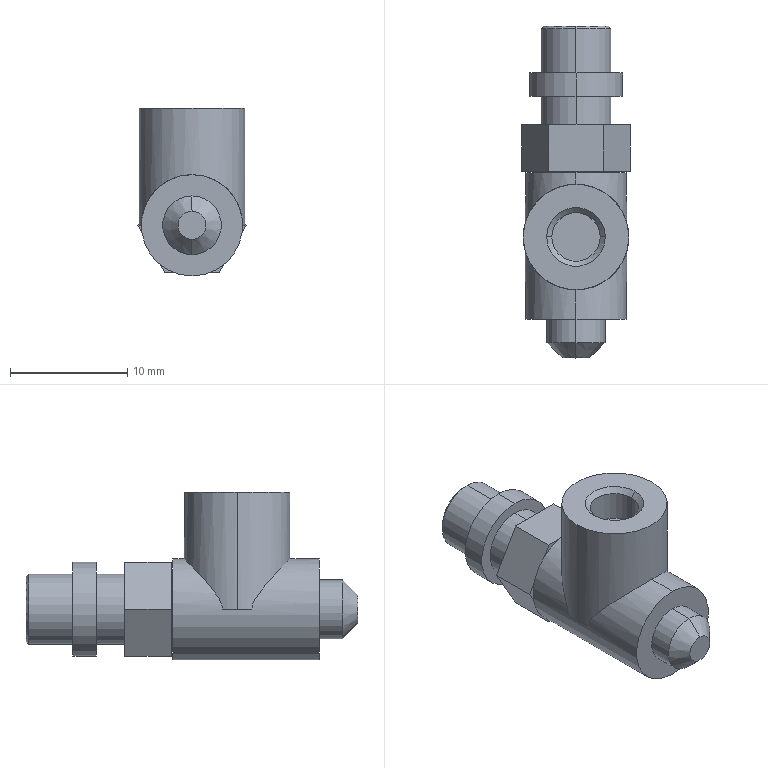Part | NX | features BREP 1 | 1 solid | 40 faces | box 9.238 x 28.3 x 14.32 mm | volume 1659 mm3 | plane 18 | cylinder 16 | cone 6 | commonest cylinder face diameters 6 x6 4.134 x2 5 x2 8 x2 8.64 x2 9 x2
STEP:
#1=CARTESIAN_POINT('',(0.,-7.,4.32));
#2=VERTEX_POINT('',#1);
#3=CARTESIAN_POINT('',(0.,-7.,-4.32));
#4=VERTEX_POINT('',#3);
#5=CARTESIAN_POINT('',(0.,-7.,0.));
#6=DIRECTION('',(0.,1.,0.));
#7=DIRECTION('',(0.,0.,1.));
#8=AXIS2_PLACEMENT_3D('',#5,#6,#7);
#9=CIRCLE('',#8,4.32);
#10=EDGE_CURVE('',#2,#4,#9,.T.);
#11=ORIENTED_EDGE('',*,*,#10,.T.);
#12=CARTESIAN_POINT('',(0.,5.5,-4.32));
#13=VERTEX_POINT('',#12);
#14=CARTESIAN_POINT('',(0.,-0.75,-4.32));
#15=DIRECTION('',(0.,1.,0.));
#16=VECTOR('',#15,1000.);
#17=LINE('',#14,#16);
#18=EDGE_CURVE('',#13,#4,#17,.F.);
#19=ORIENTED_EDGE('',*,*,#18,.F.);
#20=CARTESIAN_POINT('',(0.,5.5,4.32));
#21=VERTEX_POINT('',#20);
#22=CARTESIAN_POINT('',(0.,5.5,0.));
#23=DIRECTION('',(0.,-1.,0.));
#24=DIRECTION('',(0.,0.,1.));
#25=AXIS2_PLACEMENT_3D('',#22,#23,#24);
#26=CIRCLE('',#25,4.32);
#27=EDGE_CURVE('',#13,#21,#26,.T.);
#28=ORIENTED_EDGE('',*,*,#27,.T.);
#29=CARTESIAN_POINT('',(0.,4.5,4.32));
#30=VERTEX_POINT('',#29);
#31=CARTESIAN_POINT('',(0.,-0.75,4.32));
#32=DIRECTION('',(0.,1.,0.));
#33=VECTOR('',#32,1000.);
#34=LINE('',#31,#33);
#35=EDGE_CURVE('',#21,#30,#34,.F.);
#36=ORIENTED_EDGE('',*,*,#35,.T.);
#37=CARTESIAN_POINT('',(4.32,1.26,0.));
#38=VERTEX_POINT('',#37);
#39=CARTESIAN_POINT('',(0.,4.5,4.32));
#40=CARTESIAN_POINT('',(0.6096,4.5,4.32));
#41=CARTESIAN_POINT('',(1.582,4.292,4.104));
#42=CARTESIAN_POINT('',(2.463,3.78,3.565));
#43=CARTESIAN_POINT('',(2.856,3.486,3.251));
#44=CARTESIAN_POINT('',(3.178,3.194,2.935));
#45=CARTESIAN_POINT('',(3.354,3.002,2.726));
#46=CARTESIAN_POINT('',(3.513,2.816,2.519));
#47=CARTESIAN_POINT('',(3.649,2.634,2.314));
#48=CARTESIAN_POINT('',(3.701,2.562,2.231));
#49=CARTESIAN_POINT('',(3.832,2.363,2.001));
#50=CARTESIAN_POINT('',(3.93,2.193,1.795));
#51=CARTESIAN_POINT('',(3.983,2.097,1.678));
#52=CARTESIAN_POINT('',(4.075,1.911,1.439));
#53=CARTESIAN_POINT('',(4.137,1.773,1.252));
#54=CARTESIAN_POINT('',(4.272,1.441,0.7636));
#55=CARTESIAN_POINT('',(4.32,1.26,0.3026));
#56=CARTESIAN_POINT('',(4.32,1.26,0.));
#57=B_SPLINE_CURVE_WITH_KNOTS('',3,(#39,#40,#41,#42,#43,#44,#45,#46,#47,#48,#49,#50,#51,#52,#53,#54,#55,#56),.UNSPECIFIED.,.F.,.F.,(4,1,1,1,1,1,1,1,1,1,1,1,1,1,1,4),(0.,0.25,0.375,0.4375,0.5,0.5625,0.5938,0.625,0.6562,0.6875,0.7188,0.75,0.7812,0.8125,0.875,1.),.UNSPECIFIED.);
#58=EDGE_CURVE('',#30,#38,#57,.T.);
#59=ORIENTED_EDGE('',*,*,#58,.T.);
#60=CARTESIAN_POINT('',(4.32,-1.26,0.));
#61=VERTEX_POINT('',#60);
#62=CARTESIAN_POINT('',(4.32,-0.75,0.));
#63=DIRECTION('',(0.,-1.,0.));
#64=VECTOR('',#63,1000.);
#65=LINE('',#62,#64);
#66=EDGE_CURVE('',#38,#61,#65,.T.);
#67=ORIENTED_EDGE('',*,*,#66,.T.);
#68=CARTESIAN_POINT('',(0.,-4.5,4.32));
#69=VERTEX_POINT('',#68);
#70=CARTESIAN_POINT('',(4.32,-1.26,0.));
#71=CARTESIAN_POINT('',(4.32,-1.26,0.3026));
#72=CARTESIAN_POINT('',(4.27,-1.445,0.7694));
#73=CARTESIAN_POINT('',(4.139,-1.77,1.246));
#74=CARTESIAN_POINT('',(4.071,-1.921,1.451));
#75=CARTESIAN_POINT('',(3.984,-2.095,1.675));
#76=CARTESIAN_POINT('',(3.93,-2.193,1.795));
#77=CARTESIAN_POINT('',(3.833,-2.362,1.999));
#78=CARTESIAN_POINT('',(3.701,-2.561,2.23));
#79=CARTESIAN_POINT('',(3.649,-2.634,2.314));
#80=CARTESIAN_POINT('',(3.512,-2.817,2.52));
#81=CARTESIAN_POINT('',(3.353,-3.004,2.728));
#82=CARTESIAN_POINT('',(3.174,-3.198,2.94));
#83=CARTESIAN_POINT('',(2.854,-3.487,3.252));
#84=CARTESIAN_POINT('',(2.462,-3.781,3.565));
#85=CARTESIAN_POINT('',(1.573,-4.293,4.106));
#86=CARTESIAN_POINT('',(0.6292,-4.5,4.32));
#87=CARTESIAN_POINT('',(0.,-4.5,4.32));
#88=B_SPLINE_CURVE_WITH_KNOTS('',3,(#70,#71,#72,#73,#74,#75,#76,#77,#78,#79,#80,#81,#82,#83,#84,#85,#86,#87),.UNSPECIFIED.,.F.,.F.,(4,1,1,1,1,1,1,1,1,1,1,1,1,1,1,4),(0.,0.125,0.1875,0.2188,0.25,0.2812,0.3125,0.3438,0.375,0.4062,0.4375,0.5,0.5625,0.625,0.75,1.),.UNSPECIFIED.);
#89=EDGE_CURVE('',#61,#69,#88,.T.);
#90=ORIENTED_EDGE('',*,*,#89,.T.);
#91=CARTESIAN_POINT('',(0.,-0.75,4.32));
#92=DIRECTION('',(0.,1.,0.));
#93=VECTOR('',#92,1000.);
#94=LINE('',#91,#93);
#95=EDGE_CURVE('',#2,#69,#94,.T.);
#96=ORIENTED_EDGE('',*,*,#95,.F.);
#97=EDGE_LOOP('',(#11,#19,#28,#36,#59,#67,#90,#96));
#98=FACE_BOUND('',#97,.T.);
#99=CARTESIAN_POINT('',(0.,-0.75,0.));
#100=DIRECTION('',(0.,1.,0.));
#101=DIRECTION('',(0.,0.,1.));
#102=AXIS2_PLACEMENT_3D('',#99,#100,#101);
#103=CYLINDRICAL_SURFACE('',#102,4.32);
#104=ADVANCED_FACE('',(#98),#103,.T.);
#105=CARTESIAN_POINT('',(0.,5.5,-3.));
#106=VERTEX_POINT('',#105);
#107=CARTESIAN_POINT('',(0.,5.5,3.));
#108=VERTEX_POINT('',#107);
#109=CARTESIAN_POINT('',(0.,5.5,0.));
#110=DIRECTION('',(0.,-1.,0.));
#111=DIRECTION('',(0.,0.,1.));
#112=AXIS2_PLACEMENT_3D('',#109,#110,#111);
#113=CIRCLE('',#112,3.);
#114=EDGE_CURVE('',#106,#108,#113,.T.);
#115=ORIENTED_EDGE('',*,*,#114,.F.);
#116=CARTESIAN_POINT('',(0.,5.6,-3.));
#117=VERTEX_POINT('',#116);
#118=CARTESIAN_POINT('',(0.,8.75,-3.));
#119=DIRECTION('',(0.,1.,0.));
#120=VECTOR('',#119,1000.);
#121=LINE('',#118,#120);
#122=EDGE_CURVE('',#117,#106,#121,.F.);
#123=ORIENTED_EDGE('',*,*,#122,.F.);
#124=CARTESIAN_POINT('',(0.,5.6,3.));
#125=VERTEX_POINT('',#124);
#126=CARTESIAN_POINT('',(0.,5.6,0.));
#127=DIRECTION('',(0.,-1.,0.));
#128=DIRECTION('',(0.,0.,1.));
#129=AXIS2_PLACEMENT_3D('',#126,#127,#128);
#130=CIRCLE('',#129,3.);
#131=EDGE_CURVE('',#117,#125,#130,.T.);
#132=ORIENTED_EDGE('',*,*,#131,.T.);
#133=CARTESIAN_POINT('',(0.,8.75,3.));
#134=DIRECTION('',(0.,1.,0.));
#135=VECTOR('',#134,1000.);
#136=LINE('',#133,#135);
#137=EDGE_CURVE('',#125,#108,#136,.F.);
#138=ORIENTED_EDGE('',*,*,#137,.T.);
#139=EDGE_LOOP('',(#115,#123,#132,#138));
#140=FACE_BOUND('',#139,.T.);
#141=CARTESIAN_POINT('',(0.,8.75,0.));
#142=DIRECTION('',(0.,1.,0.));
#143=DIRECTION('',(0.,0.,1.));
#144=AXIS2_PLACEMENT_3D('',#141,#142,#143);
#145=CYLINDRICAL_SURFACE('',#144,3.);
#146=ADVANCED_FACE('',(#140),#145,.T.);
#147=CARTESIAN_POINT('',(-4.32,1.26,0.));
#148=VERTEX_POINT('',#147);
#149=CARTESIAN_POINT('',(-4.5,0.,0.));
#150=VERTEX_POINT('',#149);
#151=CARTESIAN_POINT('',(0.,0.,0.));
#152=DIRECTION('',(0.,0.,1.));
#153=DIRECTION('',(1.,0.,0.));
#154=AXIS2_PLACEMENT_3D('',#151,#152,#153);
#155=CIRCLE('',#154,4.5);
#156=EDGE_CURVE('',#148,#150,#155,.T.);
#157=ORIENTED_EDGE('',*,*,#156,.T.);
#158=CARTESIAN_POINT('',(-4.5,0.,10.));
#159=VERTEX_POINT('',#158);
#160=CARTESIAN_POINT('',(-4.5,0.,0.));
#161=DIRECTION('',(0.,0.,1.));
#162=VECTOR('',#161,1000.);
#163=LINE('',#160,#162);
#164=EDGE_CURVE('',#159,#150,#163,.F.);
#165=ORIENTED_EDGE('',*,*,#164,.F.);
#166=CARTESIAN_POINT('',(4.5,0.,10.));
#167=VERTEX_POINT('',#166);
#168=CARTESIAN_POINT('',(0.,0.,10.));
#169=DIRECTION('',(0.,0.,-1.));
#170=DIRECTION('',(1.,0.,0.));
#171=AXIS2_PLACEMENT_3D('',#168,#169,#170);
#172=CIRCLE('',#171,4.5);
#173=EDGE_CURVE('',#159,#167,#172,.T.);
#174=ORIENTED_EDGE('',*,*,#173,.T.);
#175=CARTESIAN_POINT('',(4.5,0.,0.));
#176=VERTEX_POINT('',#175);
#177=CARTESIAN_POINT('',(4.5,0.,0.));
#178=DIRECTION('',(0.,0.,1.));
#179=VECTOR('',#178,1000.);
#180=LINE('',#177,#179);
#181=EDGE_CURVE('',#167,#176,#180,.F.);
#182=ORIENTED_EDGE('',*,*,#181,.T.);
#183=CARTESIAN_POINT('',(0.,0.,0.));
#184=DIRECTION('',(0.,0.,1.));
#185=DIRECTION('',(1.,0.,0.));
#186=AXIS2_PLACEMENT_3D('',#183,#184,#185);
#187=CIRCLE('',#186,4.5);
#188=EDGE_CURVE('',#176,#38,#187,.T.);
#189=ORIENTED_EDGE('',*,*,#188,.T.);
#190=ORIENTED_EDGE('',*,*,#58,.F.);
#191=CARTESIAN_POINT('',(0.,4.5,4.32));
#192=CARTESIAN_POINT('',(-0.3068,4.5,4.32));
#193=CARTESIAN_POINT('',(-0.9138,4.443,4.26));
#194=CARTESIAN_POINT('',(-1.853,4.131,3.935));
#195=CARTESIAN_POINT('',(-2.517,3.759,3.542));
#196=CARTESIAN_POINT('',(-3.192,3.209,2.955));
#197=CARTESIAN_POINT('',(-3.655,2.651,2.336));
#198=CARTESIAN_POINT('',(-3.941,2.195,1.811));
#199=CARTESIAN_POINT('',(-4.143,1.766,1.246));
#200=CARTESIAN_POINT('',(-4.256,1.475,0.8104));
#201=CARTESIAN_POINT('',(-4.32,1.26,0.3046));
#202=CARTESIAN_POINT('',(-4.32,1.26,0.));
#203=B_SPLINE_CURVE_WITH_KNOTS('',3,(#191,#192,#193,#194,#195,#196,#197,#198,#199,#200,#201,#202),.UNSPECIFIED.,.F.,.F.,(4,1,1,1,1,1,1,1,1,4),(0.,0.125,0.25,0.375,0.5,0.625,0.75,0.8125,0.875,1.),.UNSPECIFIED.);
#204=EDGE_CURVE('',#148,#30,#203,.F.);
#205=ORIENTED_EDGE('',*,*,#204,.F.);
#206=EDGE_LOOP('',(#157,#165,#174,#182,#189,#190,#205));
#207=FACE_BOUND('',#206,.T.);
#208=CARTESIAN_POINT('',(0.,0.,0.));
#209=DIRECTION('',(0.,0.,1.));
#210=DIRECTION('',(1.,0.,0.));
#211=AXIS2_PLACEMENT_3D('',#208,#209,#210);
#212=CYLINDRICAL_SURFACE('',#211,4.5);
#213=ADVANCED_FACE('',(#207),#212,.T.);
#214=CARTESIAN_POINT('',(0.,-8.995,2.5));
#215=VERTEX_POINT('',#214);
#216=CARTESIAN_POINT('',(0.,-8.995,-2.5));
#217=VERTEX_POINT('',#216);
#218=CARTESIAN_POINT('',(0.,-8.995,0.));
#219=DIRECTION('',(0.,1.,0.));
#220=DIRECTION('',(0.,0.,1.));
#221=AXIS2_PLACEMENT_3D('',#218,#219,#220);
#222=CIRCLE('',#221,2.5);
#223=EDGE_CURVE('',#215,#217,#222,.T.);
#224=ORIENTED_EDGE('',*,*,#223,.T.);
#225=CARTESIAN_POINT('',(0.,-7.,-2.5));
#226=VERTEX_POINT('',#225);
#227=CARTESIAN_POINT('',(0.,-7.997,-2.5));
#228=DIRECTION('',(0.,1.,0.));
#229=VECTOR('',#228,1000.);
#230=LINE('',#227,#229);
#231=EDGE_CURVE('',#226,#217,#230,.F.);
#232=ORIENTED_EDGE('',*,*,#231,.F.);
#233=CARTESIAN_POINT('',(0.,-7.,2.5));
#234=VERTEX_POINT('',#233);
#235=CARTESIAN_POINT('',(0.,-7.,0.));
#236=DIRECTION('',(0.,1.,0.));
#237=DIRECTION('',(0.,0.,1.));
#238=AXIS2_PLACEMENT_3D('',#235,#236,#237);
#239=CIRCLE('',#238,2.5);
#240=EDGE_CURVE('',#234,#226,#239,.T.);
#241=ORIENTED_EDGE('',*,*,#240,.F.);
#242=CARTESIAN_POINT('',(0.,-7.997,2.5));
#243=DIRECTION('',(0.,1.,0.));
#244=VECTOR('',#243,1000.);
#245=LINE('',#242,#244);
#246=EDGE_CURVE('',#234,#215,#245,.F.);
#247=ORIENTED_EDGE('',*,*,#246,.T.);
#248=EDGE_LOOP('',(#224,#232,#241,#247));
#249=FACE_BOUND('',#248,.T.);
#250=CARTESIAN_POINT('',(0.,-7.997,0.));
#251=DIRECTION('',(0.,1.,0.));
#252=DIRECTION('',(0.,0.,1.));
#253=AXIS2_PLACEMENT_3D('',#250,#251,#252);
#254=CYLINDRICAL_SURFACE('',#253,2.5);
#255=ADVANCED_FACE('',(#249),#254,.T.);
#256=CARTESIAN_POINT('',(0.,-10.3,1.195));
#257=VERTEX_POINT('',#256);
#258=CARTESIAN_POINT('',(0.,-10.3,-1.195));
#259=VERTEX_POINT('',#258);
#260=CARTESIAN_POINT('',(0.,-10.3,0.));
#261=DIRECTION('',(0.,1.,0.));
#262=DIRECTION('',(0.,0.,1.));
#263=AXIS2_PLACEMENT_3D('',#260,#261,#262);
#264=CIRCLE('',#263,1.195);
#265=EDGE_CURVE('',#257,#259,#264,.T.);
#266=ORIENTED_EDGE('',*,*,#265,.T.);
#267=CARTESIAN_POINT('',(0.,-8.995,-2.5));
#268=DIRECTION('',(0.,0.7071,-0.7071));
#269=VECTOR('',#268,1000.);
#270=LINE('',#267,#269);
#271=EDGE_CURVE('',#217,#259,#270,.F.);
#272=ORIENTED_EDGE('',*,*,#271,.F.);
#273=ORIENTED_EDGE('',*,*,#223,.F.);
#274=CARTESIAN_POINT('',(0.,-8.995,2.5));
#275=DIRECTION('',(0.,0.7071,0.7071));
#276=VECTOR('',#275,1000.);
#277=LINE('',#274,#276);
#278=EDGE_CURVE('',#215,#257,#277,.F.);
#279=ORIENTED_EDGE('',*,*,#278,.T.);
#280=EDGE_LOOP('',(#266,#272,#273,#279));
#281=FACE_BOUND('',#280,.T.);
#282=CARTESIAN_POINT('',(0.,-8.995,0.));
#283=DIRECTION('',(0.,1.,0.));
#284=DIRECTION('',(0.,0.,1.));
#285=AXIS2_PLACEMENT_3D('',#282,#283,#284);
#286=CONICAL_SURFACE('',#285,2.5,0.7854);
#287=ADVANCED_FACE('',(#281),#286,.T.);
#288=CARTESIAN_POINT('',(-2.067,0.,9.567));
#289=VERTEX_POINT('',#288);
#290=CARTESIAN_POINT('',(2.067,0.,9.567));
#291=VERTEX_POINT('',#290);
#292=CARTESIAN_POINT('',(0.,0.,9.567));
#293=DIRECTION('',(0.,0.,1.));
#294=DIRECTION('',(0.,1.,0.));
#295=AXIS2_PLACEMENT_3D('',#292,#293,#294);
#296=CIRCLE('',#295,2.067);
#297=EDGE_CURVE('',#289,#291,#296,.T.);
#298=ORIENTED_EDGE('',*,*,#297,.F.);
#299=CARTESIAN_POINT('',(-2.5,0.,10.));
#300=VERTEX_POINT('',#299);
#301=CARTESIAN_POINT('',(-2.5,0.,10.));
#302=DIRECTION('',(-0.7071,0.,0.7071));
#303=VECTOR('',#302,1000.);
#304=LINE('',#301,#303);
#305=EDGE_CURVE('',#300,#289,#304,.F.);
#306=ORIENTED_EDGE('',*,*,#305,.F.);
#307=CARTESIAN_POINT('',(2.5,0.,10.));
#308=VERTEX_POINT('',#307);
#309=CARTESIAN_POINT('',(0.,0.,10.));
#310=DIRECTION('',(0.,0.,-1.));
#311=DIRECTION('',(1.,0.,0.));
#312=AXIS2_PLACEMENT_3D('',#309,#310,#311);
#313=CIRCLE('',#312,2.5);
#314=EDGE_CURVE('',#308,#300,#313,.T.);
#315=ORIENTED_EDGE('',*,*,#314,.F.);
#316=CARTESIAN_POINT('',(2.5,0.,10.));
#317=DIRECTION('',(0.7071,0.,0.7071));
#318=VECTOR('',#317,1000.);
#319=LINE('',#316,#318);
#320=EDGE_CURVE('',#308,#291,#319,.F.);
#321=ORIENTED_EDGE('',*,*,#320,.T.);
#322=EDGE_LOOP('',(#298,#306,#315,#321));
#323=FACE_BOUND('',#322,.T.);
#324=CARTESIAN_POINT('',(0.,0.,10.));
#325=DIRECTION('',(0.,0.,1.));
#326=DIRECTION('',(1.,0.,0.));
#327=AXIS2_PLACEMENT_3D('',#324,#325,#326);
#328=CONICAL_SURFACE('',#327,2.5,0.7854);
#329=ADVANCED_FACE('',(#323),#328,.F.);
#330=CARTESIAN_POINT('',(-2.067,0.,7.));
#331=VERTEX_POINT('',#330);
#332=CARTESIAN_POINT('',(2.067,0.,7.));
#333=VERTEX_POINT('',#332);
#334=CARTESIAN_POINT('',(0.,0.,7.));
#335=DIRECTION('',(0.,0.,1.));
#336=DIRECTION('',(1.,0.,0.));
#337=AXIS2_PLACEMENT_3D('',#334,#335,#336);
#338=CIRCLE('',#337,2.067);
#339=EDGE_CURVE('',#331,#333,#338,.T.);
#340=ORIENTED_EDGE('',*,*,#339,.F.);
#341=CARTESIAN_POINT('',(-2.067,0.,8.284));
#342=DIRECTION('',(0.,0.,1.));
#343=VECTOR('',#342,1000.);
#344=LINE('',#341,#343);
#345=EDGE_CURVE('',#289,#331,#344,.F.);
#346=ORIENTED_EDGE('',*,*,#345,.F.);
#347=ORIENTED_EDGE('',*,*,#297,.T.);
#348=CARTESIAN_POINT('',(2.067,0.,8.284));
#349=DIRECTION('',(0.,0.,1.));
#350=VECTOR('',#349,1000.);
#351=LINE('',#348,#350);
#352=EDGE_CURVE('',#291,#333,#351,.F.);
#353=ORIENTED_EDGE('',*,*,#352,.T.);
#354=EDGE_LOOP('',(#340,#346,#347,#353));
#355=FACE_BOUND('',#354,.T.);
#356=CARTESIAN_POINT('',(0.,0.,8.284));
#357=DIRECTION('',(0.,0.,1.));
#358=DIRECTION('',(1.,0.,0.));
#359=AXIS2_PLACEMENT_3D('',#356,#357,#358);
#360=CYLINDRICAL_SURFACE('',#359,2.067);
#361=ADVANCED_FACE('',(#355),#360,.F.);
#362=CARTESIAN_POINT('',(0.,9.6,-3.));
#363=VERTEX_POINT('',#362);
#364=CARTESIAN_POINT('',(0.,9.6,3.));
#365=VERTEX_POINT('',#364);
#366=CARTESIAN_POINT('',(0.,9.6,0.));
#367=DIRECTION('',(0.,-1.,0.));
#368=DIRECTION('',(0.,0.,1.));
#369=AXIS2_PLACEMENT_3D('',#366,#367,#368);
#370=CIRCLE('',#369,3.);
#371=EDGE_CURVE('',#363,#365,#370,.T.);
#372=ORIENTED_EDGE('',*,*,#371,.F.);
#373=CARTESIAN_POINT('',(0.,12.,-3.));
#374=VERTEX_POINT('',#373);
#375=CARTESIAN_POINT('',(0.,8.75,-3.));
#376=DIRECTION('',(0.,1.,0.));
#377=VECTOR('',#376,1000.);
#378=LINE('',#375,#377);
#379=EDGE_CURVE('',#374,#363,#378,.F.);
#380=ORIENTED_EDGE('',*,*,#379,.F.);
#381=CARTESIAN_POINT('',(0.,12.,3.));
#382=VERTEX_POINT('',#381);
#383=CARTESIAN_POINT('',(0.,12.,0.));
#384=DIRECTION('',(0.,-1.,0.));
#385=DIRECTION('',(0.,0.,1.));
#386=AXIS2_PLACEMENT_3D('',#383,#384,#385);
#387=CIRCLE('',#386,3.);
#388=EDGE_CURVE('',#374,#382,#387,.T.);
#389=ORIENTED_EDGE('',*,*,#388,.T.);
#390=CARTESIAN_POINT('',(0.,8.75,3.));
#391=DIRECTION('',(0.,1.,0.));
#392=VECTOR('',#391,1000.);
#393=LINE('',#390,#392);
#394=EDGE_CURVE('',#382,#365,#393,.F.);
#395=ORIENTED_EDGE('',*,*,#394,.T.);
#396=EDGE_LOOP('',(#372,#380,#389,#395));
#397=FACE_BOUND('',#396,.T.);
#398=CARTESIAN_POINT('',(0.,8.75,0.));
#399=DIRECTION('',(0.,1.,0.));
#400=DIRECTION('',(0.,0.,1.));
#401=AXIS2_PLACEMENT_3D('',#398,#399,#400);
#402=CYLINDRICAL_SURFACE('',#401,3.);
#403=ADVANCED_FACE('',(#397),#402,.T.);
#404=CARTESIAN_POINT('',(0.,12.,-4.));
#405=VERTEX_POINT('',#404);
#406=CARTESIAN_POINT('',(0.,12.,4.));
#407=VERTEX_POINT('',#406);
#408=CARTESIAN_POINT('',(0.,12.,0.));
#409=DIRECTION('',(0.,-1.,0.));
#410=DIRECTION('',(0.,0.,1.));
#411=AXIS2_PLACEMENT_3D('',#408,#409,#410);
#412=CIRCLE('',#411,4.);
#413=EDGE_CURVE('',#405,#407,#412,.T.);
#414=ORIENTED_EDGE('',*,*,#413,.F.);
#415=CARTESIAN_POINT('',(0.,14.,-4.));
#416=VERTEX_POINT('',#415);
#417=CARTESIAN_POINT('',(0.,13.,-4.));
#418=DIRECTION('',(0.,1.,0.));
#419=VECTOR('',#418,1000.);
#420=LINE('',#417,#419);
#421=EDGE_CURVE('',#416,#405,#420,.F.);
#422=ORIENTED_EDGE('',*,*,#421,.F.);
#423=CARTESIAN_POINT('',(0.,14.,4.));
#424=VERTEX_POINT('',#423);
#425=CARTESIAN_POINT('',(0.,14.,0.));
#426=DIRECTION('',(0.,-1.,0.));
#427=DIRECTION('',(0.,0.,1.));
#428=AXIS2_PLACEMENT_3D('',#425,#426,#427);
#429=CIRCLE('',#428,4.);
#430=EDGE_CURVE('',#416,#424,#429,.T.);
#431=ORIENTED_EDGE('',*,*,#430,.T.);
#432=CARTESIAN_POINT('',(0.,13.,4.));
#433=DIRECTION('',(0.,1.,0.));
#434=VECTOR('',#433,1000.);
#435=LINE('',#432,#434);
#436=EDGE_CURVE('',#424,#407,#435,.F.);
#437=ORIENTED_EDGE('',*,*,#436,.T.);
#438=EDGE_LOOP('',(#414,#422,#431,#437));
#439=FACE_BOUND('',#438,.T.);
#440=CARTESIAN_POINT('',(0.,13.,0.));
#441=DIRECTION('',(0.,1.,0.));
#442=DIRECTION('',(0.,0.,1.));
#443=AXIS2_PLACEMENT_3D('',#440,#441,#442);
#444=CYLINDRICAL_SURFACE('',#443,4.);
#445=ADVANCED_FACE('',(#439),#444,.T.);
#446=CARTESIAN_POINT('',(0.,14.,-3.));
#447=VERTEX_POINT('',#446);
#448=CARTESIAN_POINT('',(0.,14.,3.));
#449=VERTEX_POINT('',#448);
#450=CARTESIAN_POINT('',(0.,14.,0.));
#451=DIRECTION('',(0.,-1.,0.));
#452=DIRECTION('',(0.,0.,1.));
#453=AXIS2_PLACEMENT_3D('',#450,#451,#452);
#454=CIRCLE('',#453,3.);
#455=EDGE_CURVE('',#447,#449,#454,.T.);
#456=ORIENTED_EDGE('',*,*,#455,.F.);
#457=CARTESIAN_POINT('',(0.,17.767,-3.));
#458=VERTEX_POINT('',#457);
#459=CARTESIAN_POINT('',(0.,15.883,-3.));
#460=DIRECTION('',(0.,1.,0.));
#461=VECTOR('',#460,1000.);
#462=LINE('',#459,#461);
#463=EDGE_CURVE('',#458,#447,#462,.F.);
#464=ORIENTED_EDGE('',*,*,#463,.F.);
#465=CARTESIAN_POINT('',(0.,17.767,3.));
#466=VERTEX_POINT('',#465);
#467=CARTESIAN_POINT('',(0.,17.767,0.));
#468=DIRECTION('',(0.,-1.,0.));
#469=DIRECTION('',(0.,0.,1.));
#470=AXIS2_PLACEMENT_3D('',#467,#468,#469);
#471=CIRCLE('',#470,3.);
#472=EDGE_CURVE('',#458,#466,#471,.T.);
#473=ORIENTED_EDGE('',*,*,#472,.T.);
#474=CARTESIAN_POINT('',(0.,15.883,3.));
#475=DIRECTION('',(0.,1.,0.));
#476=VECTOR('',#475,1000.);
#477=LINE('',#474,#476);
#478=EDGE_CURVE('',#466,#449,#477,.F.);
#479=ORIENTED_EDGE('',*,*,#478,.T.);
#480=EDGE_LOOP('',(#456,#464,#473,#479));
#481=FACE_BOUND('',#480,.T.);
#482=CARTESIAN_POINT('',(0.,15.883,0.));
#483=DIRECTION('',(0.,1.,0.));
#484=DIRECTION('',(0.,0.,1.));
#485=AXIS2_PLACEMENT_3D('',#482,#483,#484);
#486=CYLINDRICAL_SURFACE('',#485,3.);
#487=ADVANCED_FACE('',(#481),#486,.T.);
#488=CARTESIAN_POINT('',(0.,18.,-2.767));
#489=VERTEX_POINT('',#488);
#490=CARTESIAN_POINT('',(0.,18.,2.767));
#491=VERTEX_POINT('',#490);
#492=CARTESIAN_POINT('',(0.,18.,0.));
#493=DIRECTION('',(0.,-1.,0.));
#494=DIRECTION('',(0.,0.,-1.));
#495=AXIS2_PLACEMENT_3D('',#492,#493,#494);
#496=CIRCLE('',#495,2.767);
#497=EDGE_CURVE('',#489,#491,#496,.T.);
#498=ORIENTED_EDGE('',*,*,#497,.T.);
#499=CARTESIAN_POINT('',(0.,17.767,3.));
#500=DIRECTION('',(0.,-0.7071,0.7071));
#501=VECTOR('',#500,1000.);
#502=LINE('',#499,#501);
#503=EDGE_CURVE('',#491,#466,#502,.T.);
#504=ORIENTED_EDGE('',*,*,#503,.T.);
#505=ORIENTED_EDGE('',*,*,#472,.F.);
#506=CARTESIAN_POINT('',(0.,17.767,-3.));
#507=DIRECTION('',(0.,-0.7071,-0.7071));
#508=VECTOR('',#507,1000.);
#509=LINE('',#506,#508);
#510=EDGE_CURVE('',#489,#458,#509,.T.);
#511=ORIENTED_EDGE('',*,*,#510,.F.);
#512=EDGE_LOOP('',(#498,#504,#505,#511));
#513=FACE_BOUND('',#512,.T.);
#514=CARTESIAN_POINT('',(0.,17.767,0.));
#515=DIRECTION('',(0.,-1.,0.));
#516=DIRECTION('',(0.,0.,-1.));
#517=AXIS2_PLACEMENT_3D('',#514,#515,#516);
#518=CONICAL_SURFACE('',#517,3.,0.7854);
#519=ADVANCED_FACE('',(#513),#518,.T.);
#520=ORIENTED_EDGE('',*,*,#18,.T.);
#521=CARTESIAN_POINT('',(0.,-7.,0.));
#522=DIRECTION('',(0.,1.,0.));
#523=DIRECTION('',(0.,0.,1.));
#524=AXIS2_PLACEMENT_3D('',#521,#522,#523);
#525=CIRCLE('',#524,4.32);
#526=EDGE_CURVE('',#4,#2,#525,.T.);
#527=ORIENTED_EDGE('',*,*,#526,.T.);
#528=ORIENTED_EDGE('',*,*,#95,.T.);
#529=CARTESIAN_POINT('',(-4.32,-1.26,0.));
#530=VERTEX_POINT('',#529);
#531=CARTESIAN_POINT('',(0.,-4.5,4.32));
#532=CARTESIAN_POINT('',(-0.6096,-4.5,4.32));
#533=CARTESIAN_POINT('',(-1.582,-4.292,4.104));
#534=CARTESIAN_POINT('',(-2.463,-3.78,3.565));
#535=CARTESIAN_POINT('',(-2.856,-3.486,3.251));
#536=CARTESIAN_POINT('',(-3.178,-3.194,2.935));
#537=CARTESIAN_POINT('',(-3.354,-3.002,2.726));
#538=CARTESIAN_POINT('',(-3.513,-2.816,2.519));
#539=CARTESIAN_POINT('',(-3.649,-2.634,2.314));
#540=CARTESIAN_POINT('',(-3.701,-2.562,2.231));
#541=CARTESIAN_POINT('',(-3.832,-2.363,2.001));
#542=CARTESIAN_POINT('',(-3.93,-2.193,1.795));
#543=CARTESIAN_POINT('',(-3.983,-2.097,1.678));
#544=CARTESIAN_POINT('',(-4.075,-1.911,1.439));
#545=CARTESIAN_POINT('',(-4.137,-1.773,1.252));
#546=CARTESIAN_POINT('',(-4.272,-1.441,0.7636));
#547=CARTESIAN_POINT('',(-4.32,-1.26,0.3026));
#548=CARTESIAN_POINT('',(-4.32,-1.26,0.));
#549=B_SPLINE_CURVE_WITH_KNOTS('',3,(#531,#532,#533,#534,#535,#536,#537,#538,#539,#540,#541,#542,#543,#544,#545,#546,#547,#548),.UNSPECIFIED.,.F.,.F.,(4,1,1,1,1,1,1,1,1,1,1,1,1,1,1,4),(0.,0.25,0.375,0.4375,0.5,0.5625,0.5938,0.625,0.6562,0.6875,0.7188,0.75,0.7812,0.8125,0.875,1.),.UNSPECIFIED.);
#550=EDGE_CURVE('',#69,#530,#549,.T.);
#551=ORIENTED_EDGE('',*,*,#550,.T.);
#552=CARTESIAN_POINT('',(-4.32,-0.75,0.));
#553=DIRECTION('',(0.,1.,0.));
#554=VECTOR('',#553,1000.);
#555=LINE('',#552,#554);
#556=EDGE_CURVE('',#530,#148,#555,.T.);
#557=ORIENTED_EDGE('',*,*,#556,.T.);
#558=ORIENTED_EDGE('',*,*,#204,.T.);
#559=ORIENTED_EDGE('',*,*,#35,.F.);
#560=CARTESIAN_POINT('',(0.,5.5,0.));
#561=DIRECTION('',(0.,-1.,0.));
#562=DIRECTION('',(0.,0.,1.));
#563=AXIS2_PLACEMENT_3D('',#560,#561,#562);
#564=CIRCLE('',#563,4.32);
#565=EDGE_CURVE('',#21,#13,#564,.T.);
#566=ORIENTED_EDGE('',*,*,#565,.T.);
#567=EDGE_LOOP('',(#520,#527,#528,#551,#557,#558,#559,#566));
#568=FACE_BOUND('',#567,.T.);
#569=CARTESIAN_POINT('',(0.,-0.75,0.));
#570=DIRECTION('',(0.,1.,0.));
#571=DIRECTION('',(0.,0.,1.));
#572=AXIS2_PLACEMENT_3D('',#569,#570,#571);
#573=CYLINDRICAL_SURFACE('',#572,4.32);
#574=ADVANCED_FACE('',(#568),#573,.T.);
#575=ORIENTED_EDGE('',*,*,#565,.F.);
#576=ORIENTED_EDGE('',*,*,#27,.F.);
#577=EDGE_LOOP('',(#575,#576));
#578=FACE_BOUND('',#577,.T.);
#579=CARTESIAN_POINT('',(0.,5.5,0.));
#580=DIRECTION('',(0.,-1.,0.));
#581=DIRECTION('',(0.,0.,1.));
#582=AXIS2_PLACEMENT_3D('',#579,#580,#581);
#583=CIRCLE('',#582,3.);
#584=EDGE_CURVE('',#108,#106,#583,.T.);
#585=ORIENTED_EDGE('',*,*,#584,.T.);
#586=ORIENTED_EDGE('',*,*,#114,.T.);
#587=EDGE_LOOP('',(#585,#586));
#588=FACE_BOUND('',#587,.T.);
#589=CARTESIAN_POINT('',(3.66,5.5,0.));
#590=DIRECTION('',(0.,1.,0.));
#591=DIRECTION('',(1.,0.,0.));
#592=AXIS2_PLACEMENT_3D('',#589,#590,#591);
#593=PLANE('',#592);
#594=ADVANCED_FACE('',(#578,#588),#593,.T.);
#595=ORIENTED_EDGE('',*,*,#556,.F.);
#596=CARTESIAN_POINT('',(0.,0.,0.));
#597=DIRECTION('',(0.,0.,1.));
#598=DIRECTION('',(1.,0.,0.));
#599=AXIS2_PLACEMENT_3D('',#596,#597,#598);
#600=CIRCLE('',#599,4.5);
#601=EDGE_CURVE('',#150,#530,#600,.T.);
#602=ORIENTED_EDGE('',*,*,#601,.F.);
#603=ORIENTED_EDGE('',*,*,#156,.F.);
#604=EDGE_LOOP('',(#595,#602,#603));
#605=FACE_BOUND('',#604,.T.);
#606=CARTESIAN_POINT('',(0.,0.,0.));
#607=DIRECTION('',(0.,0.,1.));
#608=DIRECTION('',(1.,0.,0.));
#609=AXIS2_PLACEMENT_3D('',#606,#607,#608);
#610=PLANE('',#609);
#611=ADVANCED_FACE('',(#605),#610,.F.);
#612=ORIENTED_EDGE('',*,*,#10,.F.);
#613=ORIENTED_EDGE('',*,*,#526,.F.);
#614=EDGE_LOOP('',(#612,#613));
#615=FACE_BOUND('',#614,.T.);
#616=ORIENTED_EDGE('',*,*,#240,.T.);
#617=CARTESIAN_POINT('',(0.,-7.,0.));
#618=DIRECTION('',(0.,1.,0.));
#619=DIRECTION('',(0.,0.,1.));
#620=AXIS2_PLACEMENT_3D('',#617,#618,#619);
#621=CIRCLE('',#620,2.5);
#622=EDGE_CURVE('',#226,#234,#621,.T.);
#623=ORIENTED_EDGE('',*,*,#622,.T.);
#624=EDGE_LOOP('',(#616,#623));
#625=FACE_BOUND('',#624,.T.);
#626=CARTESIAN_POINT('',(3.41,-7.,0.));
#627=DIRECTION('',(0.,-1.,0.));
#628=DIRECTION('',(-1.,0.,0.));
#629=AXIS2_PLACEMENT_3D('',#626,#627,#628);
#630=PLANE('',#629);
#631=ADVANCED_FACE('',(#615,#625),#630,.T.);
#632=CARTESIAN_POINT('',(0.,0.,0.));
#633=DIRECTION('',(0.,0.,1.));
#634=DIRECTION('',(1.,0.,0.));
#635=AXIS2_PLACEMENT_3D('',#632,#633,#634);
#636=CIRCLE('',#635,4.5);
#637=EDGE_CURVE('',#61,#176,#636,.T.);
#638=ORIENTED_EDGE('',*,*,#637,.F.);
#639=ORIENTED_EDGE('',*,*,#66,.F.);
#640=ORIENTED_EDGE('',*,*,#188,.F.);
#641=EDGE_LOOP('',(#638,#639,#640));
#642=FACE_BOUND('',#641,.T.);
#643=CARTESIAN_POINT('',(0.,0.,0.));
#644=DIRECTION('',(0.,0.,1.));
#645=DIRECTION('',(1.,0.,0.));
#646=AXIS2_PLACEMENT_3D('',#643,#644,#645);
#647=PLANE('',#646);
#648=ADVANCED_FACE('',(#642),#647,.F.);
#649=ORIENTED_EDGE('',*,*,#122,.T.);
#650=ORIENTED_EDGE('',*,*,#584,.F.);
#651=ORIENTED_EDGE('',*,*,#137,.F.);
#652=CARTESIAN_POINT('',(0.,5.6,0.));
#653=DIRECTION('',(0.,-1.,0.));
#654=DIRECTION('',(0.,0.,1.));
#655=AXIS2_PLACEMENT_3D('',#652,#653,#654);
#656=CIRCLE('',#655,3.);
#657=EDGE_CURVE('',#125,#117,#656,.T.);
#658=ORIENTED_EDGE('',*,*,#657,.T.);
#659=EDGE_LOOP('',(#649,#650,#651,#658));
#660=FACE_BOUND('',#659,.T.);
#661=CARTESIAN_POINT('',(0.,8.75,0.));
#662=DIRECTION('',(0.,1.,0.));
#663=DIRECTION('',(0.,0.,1.));
#664=AXIS2_PLACEMENT_3D('',#661,#662,#663);
#665=CYLINDRICAL_SURFACE('',#664,3.);
#666=ADVANCED_FACE('',(#660),#665,.T.);
#667=ORIENTED_EDGE('',*,*,#164,.T.);
#668=ORIENTED_EDGE('',*,*,#601,.T.);
#669=ORIENTED_EDGE('',*,*,#550,.F.);
#670=ORIENTED_EDGE('',*,*,#89,.F.);
#671=ORIENTED_EDGE('',*,*,#637,.T.);
#672=ORIENTED_EDGE('',*,*,#181,.F.);
#673=CARTESIAN_POINT('',(0.,0.,10.));
#674=DIRECTION('',(0.,0.,-1.));
#675=DIRECTION('',(1.,0.,0.));
#676=AXIS2_PLACEMENT_3D('',#673,#674,#675);
#677=CIRCLE('',#676,4.5);
#678=EDGE_CURVE('',#167,#159,#677,.T.);
#679=ORIENTED_EDGE('',*,*,#678,.T.);
#680=EDGE_LOOP('',(#667,#668,#669,#670,#671,#672,#679));
#681=FACE_BOUND('',#680,.T.);
#682=CARTESIAN_POINT('',(0.,0.,0.));
#683=DIRECTION('',(0.,0.,1.));
#684=DIRECTION('',(1.,0.,0.));
#685=AXIS2_PLACEMENT_3D('',#682,#683,#684);
#686=CYLINDRICAL_SURFACE('',#685,4.5);
#687=ADVANCED_FACE('',(#681),#686,.T.);
#688=ORIENTED_EDGE('',*,*,#231,.T.);
#689=CARTESIAN_POINT('',(0.,-8.995,0.));
#690=DIRECTION('',(0.,1.,0.));
#691=DIRECTION('',(0.,0.,1.));
#692=AXIS2_PLACEMENT_3D('',#689,#690,#691);
#693=CIRCLE('',#692,2.5);
#694=EDGE_CURVE('',#217,#215,#693,.T.);
#695=ORIENTED_EDGE('',*,*,#694,.T.);
#696=ORIENTED_EDGE('',*,*,#246,.F.);
#697=ORIENTED_EDGE('',*,*,#622,.F.);
#698=EDGE_LOOP('',(#688,#695,#696,#697));
#699=FACE_BOUND('',#698,.T.);
#700=CARTESIAN_POINT('',(0.,-7.997,0.));
#701=DIRECTION('',(0.,1.,0.));
#702=DIRECTION('',(0.,0.,1.));
#703=AXIS2_PLACEMENT_3D('',#700,#701,#702);
#704=CYLINDRICAL_SURFACE('',#703,2.5);
#705=ADVANCED_FACE('',(#699),#704,.T.);
#706=CARTESIAN_POINT('',(-2.309,5.6,-4.));
#707=VERTEX_POINT('',#706);
#708=CARTESIAN_POINT('',(-4.619,5.6,0.));
#709=VERTEX_POINT('',#708);
#710=CARTESIAN_POINT('',(-2.309,5.6,-4.));
#711=DIRECTION('',(-0.5,0.,0.866));
#712=VECTOR('',#711,1000.);
#713=LINE('',#710,#712);
#714=EDGE_CURVE('',#707,#709,#713,.T.);
#715=ORIENTED_EDGE('',*,*,#714,.F.);
#716=CARTESIAN_POINT('',(2.309,5.6,-4.));
#717=VERTEX_POINT('',#716);
#718=CARTESIAN_POINT('',(0.,5.6,-4.));
#719=DIRECTION('',(-1.,0.,0.));
#720=VECTOR('',#719,1000.);
#721=LINE('',#718,#720);
#722=EDGE_CURVE('',#717,#707,#721,.T.);
#723=ORIENTED_EDGE('',*,*,#722,.F.);
#724=CARTESIAN_POINT('',(4.619,5.6,0.));
#725=VERTEX_POINT('',#724);
#726=CARTESIAN_POINT('',(4.619,5.6,0.));
#727=DIRECTION('',(-0.5,0.,-0.866));
#728=VECTOR('',#727,1000.);
#729=LINE('',#726,#728);
#730=EDGE_CURVE('',#725,#717,#729,.T.);
#731=ORIENTED_EDGE('',*,*,#730,.F.);
#732=CARTESIAN_POINT('',(2.309,5.6,4.));
#733=VERTEX_POINT('',#732);
#734=CARTESIAN_POINT('',(2.309,5.6,4.));
#735=DIRECTION('',(0.5,0.,-0.866));
#736=VECTOR('',#735,1000.);
#737=LINE('',#734,#736);
#738=EDGE_CURVE('',#733,#725,#737,.T.);
#739=ORIENTED_EDGE('',*,*,#738,.F.);
#740=CARTESIAN_POINT('',(-2.309,5.6,4.));
#741=VERTEX_POINT('',#740);
#742=CARTESIAN_POINT('',(0.,5.6,4.));
#743=DIRECTION('',(1.,0.,0.));
#744=VECTOR('',#743,1000.);
#745=LINE('',#742,#744);
#746=EDGE_CURVE('',#741,#733,#745,.T.);
#747=ORIENTED_EDGE('',*,*,#746,.F.);
#748=CARTESIAN_POINT('',(-4.619,5.6,0.));
#749=DIRECTION('',(0.5,0.,0.866));
#750=VECTOR('',#749,1000.);
#751=LINE('',#748,#750);
#752=EDGE_CURVE('',#709,#741,#751,.T.);
#753=ORIENTED_EDGE('',*,*,#752,.F.);
#754=EDGE_LOOP('',(#715,#723,#731,#739,#747,#753));
#755=FACE_BOUND('',#754,.T.);
#756=ORIENTED_EDGE('',*,*,#657,.F.);
#757=ORIENTED_EDGE('',*,*,#131,.F.);
#758=EDGE_LOOP('',(#756,#757));
#759=FACE_BOUND('',#758,.T.);
#760=CARTESIAN_POINT('',(0.,5.6,0.));
#761=DIRECTION('',(0.,1.,0.));
#762=DIRECTION('',(1.,0.,0.));
#763=AXIS2_PLACEMENT_3D('',#760,#761,#762);
#764=PLANE('',#763);
#765=ADVANCED_FACE('',(#755,#759),#764,.F.);
#766=ORIENTED_EDGE('',*,*,#678,.F.);
#767=ORIENTED_EDGE('',*,*,#173,.F.);
#768=EDGE_LOOP('',(#766,#767));
#769=FACE_BOUND('',#768,.T.);
#770=ORIENTED_EDGE('',*,*,#314,.T.);
#771=CARTESIAN_POINT('',(0.,0.,10.));
#772=DIRECTION('',(0.,0.,-1.));
#773=DIRECTION('',(1.,0.,0.));
#774=AXIS2_PLACEMENT_3D('',#771,#772,#773);
#775=CIRCLE('',#774,2.5);
#776=EDGE_CURVE('',#300,#308,#775,.T.);
#777=ORIENTED_EDGE('',*,*,#776,.T.);
#778=EDGE_LOOP('',(#770,#777));
#779=FACE_BOUND('',#778,.T.);
#780=CARTESIAN_POINT('',(0.,0.,10.));
#781=DIRECTION('',(0.,0.,1.));
#782=DIRECTION('',(1.,0.,0.));
#783=AXIS2_PLACEMENT_3D('',#780,#781,#782);
#784=PLANE('',#783);
#785=ADVANCED_FACE('',(#769,#779),#784,.T.);
#786=ORIENTED_EDGE('',*,*,#271,.T.);
#787=CARTESIAN_POINT('',(0.,-10.3,0.));
#788=DIRECTION('',(0.,1.,0.));
#789=DIRECTION('',(0.,0.,1.));
#790=AXIS2_PLACEMENT_3D('',#787,#788,#789);
#791=CIRCLE('',#790,1.195);
#792=EDGE_CURVE('',#259,#257,#791,.T.);
#793=ORIENTED_EDGE('',*,*,#792,.T.);
#794=ORIENTED_EDGE('',*,*,#278,.F.);
#795=ORIENTED_EDGE('',*,*,#694,.F.);
#796=EDGE_LOOP('',(#786,#793,#794,#795));
#797=FACE_BOUND('',#796,.T.);
#798=CARTESIAN_POINT('',(0.,-8.995,0.));
#799=DIRECTION('',(0.,1.,0.));
#800=DIRECTION('',(0.,0.,1.));
#801=AXIS2_PLACEMENT_3D('',#798,#799,#800);
#802=CONICAL_SURFACE('',#801,2.5,0.7854);
#803=ADVANCED_FACE('',(#797),#802,.T.);
#804=ORIENTED_EDGE('',*,*,#752,.T.);
#805=CARTESIAN_POINT('',(-2.309,9.6,4.));
#806=VERTEX_POINT('',#805);
#807=CARTESIAN_POINT('',(-2.309,5.6,4.));
#808=DIRECTION('',(0.,1.,0.));
#809=VECTOR('',#808,1000.);
#810=LINE('',#807,#809);
#811=EDGE_CURVE('',#741,#806,#810,.T.);
#812=ORIENTED_EDGE('',*,*,#811,.T.);
#813=CARTESIAN_POINT('',(-4.619,9.6,0.));
#814=VERTEX_POINT('',#813);
#815=CARTESIAN_POINT('',(-2.309,9.6,4.));
#816=DIRECTION('',(-0.5,0.,-0.866));
#817=VECTOR('',#816,1000.);
#818=LINE('',#815,#817);
#819=EDGE_CURVE('',#806,#814,#818,.T.);
#820=ORIENTED_EDGE('',*,*,#819,.T.);
#821=CARTESIAN_POINT('',(-4.619,5.6,0.));
#822=DIRECTION('',(0.,-1.,0.));
#823=VECTOR('',#822,1000.);
#824=LINE('',#821,#823);
#825=EDGE_CURVE('',#814,#709,#824,.T.);
#826=ORIENTED_EDGE('',*,*,#825,.T.);
#827=EDGE_LOOP('',(#804,#812,#820,#826));
#828=FACE_BOUND('',#827,.T.);
#829=CARTESIAN_POINT('',(-2.309,5.6,4.));
#830=DIRECTION('',(-0.866,0.,0.5));
#831=DIRECTION('',(0.,1.,0.));
#832=AXIS2_PLACEMENT_3D('',#829,#830,#831);
#833=PLANE('',#832);
#834=ADVANCED_FACE('',(#828),#833,.T.);
#835=ORIENTED_EDGE('',*,*,#714,.T.);
#836=ORIENTED_EDGE('',*,*,#825,.F.);
#837=CARTESIAN_POINT('',(-2.309,9.6,-4.));
#838=VERTEX_POINT('',#837);
#839=CARTESIAN_POINT('',(-4.619,9.6,0.));
#840=DIRECTION('',(0.5,0.,-0.866));
#841=VECTOR('',#840,1000.);
#842=LINE('',#839,#841);
#843=EDGE_CURVE('',#814,#838,#842,.T.);
#844=ORIENTED_EDGE('',*,*,#843,.T.);
#845=CARTESIAN_POINT('',(-2.309,5.6,-4.));
#846=DIRECTION('',(0.,-1.,0.));
#847=VECTOR('',#846,1000.);
#848=LINE('',#845,#847);
#849=EDGE_CURVE('',#838,#707,#848,.T.);
#850=ORIENTED_EDGE('',*,*,#849,.T.);
#851=EDGE_LOOP('',(#835,#836,#844,#850));
#852=FACE_BOUND('',#851,.T.);
#853=CARTESIAN_POINT('',(-4.619,5.6,0.));
#854=DIRECTION('',(-0.866,0.,-0.5));
#855=DIRECTION('',(-0.5,0.,0.866));
#856=AXIS2_PLACEMENT_3D('',#853,#854,#855);
#857=PLANE('',#856);
#858=ADVANCED_FACE('',(#852),#857,.T.);
#859=ORIENTED_EDGE('',*,*,#722,.T.);
#860=ORIENTED_EDGE('',*,*,#849,.F.);
#861=CARTESIAN_POINT('',(2.309,9.6,-4.));
#862=VERTEX_POINT('',#861);
#863=CARTESIAN_POINT('',(-2.309,9.6,-4.));
#864=DIRECTION('',(1.,0.,0.));
#865=VECTOR('',#864,1000.);
#866=LINE('',#863,#865);
#867=EDGE_CURVE('',#838,#862,#866,.T.);
#868=ORIENTED_EDGE('',*,*,#867,.T.);
#869=CARTESIAN_POINT('',(2.309,5.6,-4.));
#870=DIRECTION('',(0.,-1.,0.));
#871=VECTOR('',#870,1000.);
#872=LINE('',#869,#871);
#873=EDGE_CURVE('',#862,#717,#872,.T.);
#874=ORIENTED_EDGE('',*,*,#873,.T.);
#875=EDGE_LOOP('',(#859,#860,#868,#874));
#876=FACE_BOUND('',#875,.T.);
#877=CARTESIAN_POINT('',(-2.309,5.6,-4.));
#878=DIRECTION('',(0.,0.,-1.));
#879=DIRECTION('',(-1.,0.,0.));
#880=AXIS2_PLACEMENT_3D('',#877,#878,#879);
#881=PLANE('',#880);
#882=ADVANCED_FACE('',(#876),#881,.T.);
#883=ORIENTED_EDGE('',*,*,#730,.T.);
#884=ORIENTED_EDGE('',*,*,#873,.F.);
#885=CARTESIAN_POINT('',(4.619,9.6,0.));
#886=VERTEX_POINT('',#885);
#887=CARTESIAN_POINT('',(2.309,9.6,-4.));
#888=DIRECTION('',(0.5,0.,0.866));
#889=VECTOR('',#888,1000.);
#890=LINE('',#887,#889);
#891=EDGE_CURVE('',#862,#886,#890,.T.);
#892=ORIENTED_EDGE('',*,*,#891,.T.);
#893=CARTESIAN_POINT('',(4.619,5.6,0.));
#894=DIRECTION('',(0.,-1.,0.));
#895=VECTOR('',#894,1000.);
#896=LINE('',#893,#895);
#897=EDGE_CURVE('',#886,#725,#896,.T.);
#898=ORIENTED_EDGE('',*,*,#897,.T.);
#899=EDGE_LOOP('',(#883,#884,#892,#898));
#900=FACE_BOUND('',#899,.T.);
#901=CARTESIAN_POINT('',(2.309,5.6,-4.));
#902=DIRECTION('',(0.866,0.,-0.5));
#903=DIRECTION('',(0.,-1.,0.));
#904=AXIS2_PLACEMENT_3D('',#901,#902,#903);
#905=PLANE('',#904);
#906=ADVANCED_FACE('',(#900),#905,.T.);
#907=ORIENTED_EDGE('',*,*,#738,.T.);
#908=ORIENTED_EDGE('',*,*,#897,.F.);
#909=CARTESIAN_POINT('',(2.309,9.6,4.));
#910=VERTEX_POINT('',#909);
#911=CARTESIAN_POINT('',(4.619,9.6,0.));
#912=DIRECTION('',(-0.5,0.,0.866));
#913=VECTOR('',#912,1000.);
#914=LINE('',#911,#913);
#915=EDGE_CURVE('',#886,#910,#914,.T.);
#916=ORIENTED_EDGE('',*,*,#915,.T.);
#917=CARTESIAN_POINT('',(2.309,5.6,4.));
#918=DIRECTION('',(0.,-1.,0.));
#919=VECTOR('',#918,1000.);
#920=LINE('',#917,#919);
#921=EDGE_CURVE('',#910,#733,#920,.T.);
#922=ORIENTED_EDGE('',*,*,#921,.T.);
#923=EDGE_LOOP('',(#907,#908,#916,#922));
#924=FACE_BOUND('',#923,.T.);
#925=CARTESIAN_POINT('',(4.619,5.6,0.));
#926=DIRECTION('',(0.866,0.,0.5));
#927=DIRECTION('',(0.,-1.,0.));
#928=AXIS2_PLACEMENT_3D('',#925,#926,#927);
#929=PLANE('',#928);
#930=ADVANCED_FACE('',(#924),#929,.T.);
#931=ORIENTED_EDGE('',*,*,#746,.T.);
#932=ORIENTED_EDGE('',*,*,#921,.F.);
#933=CARTESIAN_POINT('',(2.309,9.6,4.));
#934=DIRECTION('',(-1.,0.,0.));
#935=VECTOR('',#934,1000.);
#936=LINE('',#933,#935);
#937=EDGE_CURVE('',#910,#806,#936,.T.);
#938=ORIENTED_EDGE('',*,*,#937,.T.);
#939=ORIENTED_EDGE('',*,*,#811,.F.);
#940=EDGE_LOOP('',(#931,#932,#938,#939));
#941=FACE_BOUND('',#940,.T.);
#942=CARTESIAN_POINT('',(2.309,5.6,4.));
#943=DIRECTION('',(0.,0.,1.));
#944=DIRECTION('',(1.,0.,0.));
#945=AXIS2_PLACEMENT_3D('',#942,#943,#944);
#946=PLANE('',#945);
#947=ADVANCED_FACE('',(#941),#946,.T.);
#948=ORIENTED_EDGE('',*,*,#305,.T.);
#949=CARTESIAN_POINT('',(0.,0.,9.567));
#950=DIRECTION('',(0.,0.,1.));
#951=DIRECTION('',(0.,1.,0.));
#952=AXIS2_PLACEMENT_3D('',#949,#950,#951);
#953=CIRCLE('',#952,2.067);
#954=EDGE_CURVE('',#291,#289,#953,.T.);
#955=ORIENTED_EDGE('',*,*,#954,.F.);
#956=ORIENTED_EDGE('',*,*,#320,.F.);
#957=ORIENTED_EDGE('',*,*,#776,.F.);
#958=EDGE_LOOP('',(#948,#955,#956,#957));
#959=FACE_BOUND('',#958,.T.);
#960=CARTESIAN_POINT('',(0.,0.,10.));
#961=DIRECTION('',(0.,0.,1.));
#962=DIRECTION('',(1.,0.,0.));
#963=AXIS2_PLACEMENT_3D('',#960,#961,#962);
#964=CONICAL_SURFACE('',#963,2.5,0.7854);
#965=ADVANCED_FACE('',(#959),#964,.F.);
#966=ORIENTED_EDGE('',*,*,#265,.F.);
#967=ORIENTED_EDGE('',*,*,#792,.F.);
#968=EDGE_LOOP('',(#966,#967));
#969=FACE_BOUND('',#968,.T.);
#970=CARTESIAN_POINT('',(0.5975,-10.3,0.));
#971=DIRECTION('',(0.,-1.,0.));
#972=DIRECTION('',(-1.,0.,0.));
#973=AXIS2_PLACEMENT_3D('',#970,#971,#972);
#974=PLANE('',#973);
#975=ADVANCED_FACE('',(#969),#974,.T.);
#976=ORIENTED_EDGE('',*,*,#891,.F.);
#977=ORIENTED_EDGE('',*,*,#867,.F.);
#978=ORIENTED_EDGE('',*,*,#843,.F.);
#979=ORIENTED_EDGE('',*,*,#819,.F.);
#980=ORIENTED_EDGE('',*,*,#937,.F.);
#981=ORIENTED_EDGE('',*,*,#915,.F.);
#982=EDGE_LOOP('',(#976,#977,#978,#979,#980,#981));
#983=FACE_BOUND('',#982,.T.);
#984=CARTESIAN_POINT('',(0.,9.6,0.));
#985=DIRECTION('',(0.,-1.,0.));
#986=DIRECTION('',(0.,0.,1.));
#987=AXIS2_PLACEMENT_3D('',#984,#985,#986);
#988=CIRCLE('',#987,3.);
#989=EDGE_CURVE('',#365,#363,#988,.T.);
#990=ORIENTED_EDGE('',*,*,#989,.T.);
#991=ORIENTED_EDGE('',*,*,#371,.T.);
#992=EDGE_LOOP('',(#990,#991));
#993=FACE_BOUND('',#992,.T.);
#994=CARTESIAN_POINT('',(0.,9.6,0.));
#995=DIRECTION('',(0.,1.,0.));
#996=DIRECTION('',(1.,0.,0.));
#997=AXIS2_PLACEMENT_3D('',#994,#995,#996);
#998=PLANE('',#997);
#999=ADVANCED_FACE('',(#983,#993),#998,.T.);
#1000=ORIENTED_EDGE('',*,*,#345,.T.);
#1001=CARTESIAN_POINT('',(0.,0.,7.));
#1002=DIRECTION('',(0.,0.,1.));
#1003=DIRECTION('',(1.,0.,0.));
#1004=AXIS2_PLACEMENT_3D('',#1001,#1002,#1003);
#1005=CIRCLE('',#1004,2.067);
#1006=EDGE_CURVE('',#333,#331,#1005,.T.);
#1007=ORIENTED_EDGE('',*,*,#1006,.F.);
#1008=ORIENTED_EDGE('',*,*,#352,.F.);
#1009=ORIENTED_EDGE('',*,*,#954,.T.);
#1010=EDGE_LOOP('',(#1000,#1007,#1008,#1009));
#1011=FACE_BOUND('',#1010,.T.);
#1012=CARTESIAN_POINT('',(0.,0.,8.284));
#1013=DIRECTION('',(0.,0.,1.));
#1014=DIRECTION('',(1.,0.,0.));
#1015=AXIS2_PLACEMENT_3D('',#1012,#1013,#1014);
#1016=CYLINDRICAL_SURFACE('',#1015,2.067);
#1017=ADVANCED_FACE('',(#1011),#1016,.F.);
#1018=ORIENTED_EDGE('',*,*,#379,.T.);
#1019=ORIENTED_EDGE('',*,*,#989,.F.);
#1020=ORIENTED_EDGE('',*,*,#394,.F.);
#1021=CARTESIAN_POINT('',(0.,12.,0.));
#1022=DIRECTION('',(0.,-1.,0.));
#1023=DIRECTION('',(0.,0.,1.));
#1024=AXIS2_PLACEMENT_3D('',#1021,#1022,#1023);
#1025=CIRCLE('',#1024,3.);
#1026=EDGE_CURVE('',#382,#374,#1025,.T.);
#1027=ORIENTED_EDGE('',*,*,#1026,.T.);
#1028=EDGE_LOOP('',(#1018,#1019,#1020,#1027));
#1029=FACE_BOUND('',#1028,.T.);
#1030=CARTESIAN_POINT('',(0.,8.75,0.));
#1031=DIRECTION('',(0.,1.,0.));
#1032=DIRECTION('',(0.,0.,1.));
#1033=AXIS2_PLACEMENT_3D('',#1030,#1031,#1032);
#1034=CYLINDRICAL_SURFACE('',#1033,3.);
#1035=ADVANCED_FACE('',(#1029),#1034,.T.);
#1036=ORIENTED_EDGE('',*,*,#1006,.T.);
#1037=ORIENTED_EDGE('',*,*,#339,.T.);
#1038=EDGE_LOOP('',(#1036,#1037));
#1039=FACE_BOUND('',#1038,.T.);
#1040=CARTESIAN_POINT('',(0.,1.034,7.));
#1041=DIRECTION('',(0.,0.,-1.));
#1042=DIRECTION('',(-1.,0.,0.));
#1043=AXIS2_PLACEMENT_3D('',#1040,#1041,#1042);
#1044=PLANE('',#1043);
#1045=ADVANCED_FACE('',(#1039),#1044,.F.);
#1046=CARTESIAN_POINT('',(0.,12.,0.));
#1047=DIRECTION('',(0.,-1.,0.));
#1048=DIRECTION('',(0.,0.,1.));
#1049=AXIS2_PLACEMENT_3D('',#1046,#1047,#1048);
#1050=CIRCLE('',#1049,4.);
#1051=EDGE_CURVE('',#407,#405,#1050,.T.);
#1052=ORIENTED_EDGE('',*,*,#1051,.T.);
#1053=ORIENTED_EDGE('',*,*,#413,.T.);
#1054=EDGE_LOOP('',(#1052,#1053));
#1055=FACE_BOUND('',#1054,.T.);
#1056=ORIENTED_EDGE('',*,*,#1026,.F.);
#1057=ORIENTED_EDGE('',*,*,#388,.F.);
#1058=EDGE_LOOP('',(#1056,#1057));
#1059=FACE_BOUND('',#1058,.T.);
#1060=CARTESIAN_POINT('',(3.5,12.,0.));
#1061=DIRECTION('',(0.,-1.,0.));
#1062=DIRECTION('',(-1.,0.,0.));
#1063=AXIS2_PLACEMENT_3D('',#1060,#1061,#1062);
#1064=PLANE('',#1063);
#1065=ADVANCED_FACE('',(#1055,#1059),#1064,.T.);
#1066=ORIENTED_EDGE('',*,*,#421,.T.);
#1067=ORIENTED_EDGE('',*,*,#1051,.F.);
#1068=ORIENTED_EDGE('',*,*,#436,.F.);
#1069=CARTESIAN_POINT('',(0.,14.,0.));
#1070=DIRECTION('',(0.,-1.,0.));
#1071=DIRECTION('',(0.,0.,1.));
#1072=AXIS2_PLACEMENT_3D('',#1069,#1070,#1071);
#1073=CIRCLE('',#1072,4.);
#1074=EDGE_CURVE('',#424,#416,#1073,.T.);
#1075=ORIENTED_EDGE('',*,*,#1074,.T.);
#1076=EDGE_LOOP('',(#1066,#1067,#1068,#1075));
#1077=FACE_BOUND('',#1076,.T.);
#1078=CARTESIAN_POINT('',(0.,13.,0.));
#1079=DIRECTION('',(0.,1.,0.));
#1080=DIRECTION('',(0.,0.,1.));
#1081=AXIS2_PLACEMENT_3D('',#1078,#1079,#1080);
#1082=CYLINDRICAL_SURFACE('',#1081,4.);
#1083=ADVANCED_FACE('',(#1077),#1082,.T.);
#1084=ORIENTED_EDGE('',*,*,#1074,.F.);
#1085=ORIENTED_EDGE('',*,*,#430,.F.);
#1086=EDGE_LOOP('',(#1084,#1085));
#1087=FACE_BOUND('',#1086,.T.);
#1088=CARTESIAN_POINT('',(0.,14.,0.));
#1089=DIRECTION('',(0.,-1.,0.));
#1090=DIRECTION('',(0.,0.,1.));
#1091=AXIS2_PLACEMENT_3D('',#1088,#1089,#1090);
#1092=CIRCLE('',#1091,3.);
#1093=EDGE_CURVE('',#449,#447,#1092,.T.);
#1094=ORIENTED_EDGE('',*,*,#1093,.T.);
#1095=ORIENTED_EDGE('',*,*,#455,.T.);
#1096=EDGE_LOOP('',(#1094,#1095));
#1097=FACE_BOUND('',#1096,.T.);
#1098=CARTESIAN_POINT('',(3.5,14.,0.));
#1099=DIRECTION('',(0.,1.,0.));
#1100=DIRECTION('',(1.,0.,0.));
#1101=AXIS2_PLACEMENT_3D('',#1098,#1099,#1100);
#1102=PLANE('',#1101);
#1103=ADVANCED_FACE('',(#1087,#1097),#1102,.T.);
#1104=ORIENTED_EDGE('',*,*,#463,.T.);
#1105=ORIENTED_EDGE('',*,*,#1093,.F.);
#1106=ORIENTED_EDGE('',*,*,#478,.F.);
#1107=CARTESIAN_POINT('',(0.,17.767,0.));
#1108=DIRECTION('',(0.,-1.,0.));
#1109=DIRECTION('',(0.,0.,1.));
#1110=AXIS2_PLACEMENT_3D('',#1107,#1108,#1109);
#1111=CIRCLE('',#1110,3.);
#1112=EDGE_CURVE('',#466,#458,#1111,.T.);
#1113=ORIENTED_EDGE('',*,*,#1112,.T.);
#1114=EDGE_LOOP('',(#1104,#1105,#1106,#1113));
#1115=FACE_BOUND('',#1114,.T.);
#1116=CARTESIAN_POINT('',(0.,15.883,0.));
#1117=DIRECTION('',(0.,1.,0.));
#1118=DIRECTION('',(0.,0.,1.));
#1119=AXIS2_PLACEMENT_3D('',#1116,#1117,#1118);
#1120=CYLINDRICAL_SURFACE('',#1119,3.);
#1121=ADVANCED_FACE('',(#1115),#1120,.T.);
#1122=ORIENTED_EDGE('',*,*,#503,.F.);
#1123=CARTESIAN_POINT('',(0.,18.,0.));
#1124=DIRECTION('',(0.,-1.,0.));
#1125=DIRECTION('',(0.,0.,-1.));
#1126=AXIS2_PLACEMENT_3D('',#1123,#1124,#1125);
#1127=CIRCLE('',#1126,2.767);
#1128=EDGE_CURVE('',#491,#489,#1127,.T.);
#1129=ORIENTED_EDGE('',*,*,#1128,.T.);
#1130=ORIENTED_EDGE('',*,*,#510,.T.);
#1131=ORIENTED_EDGE('',*,*,#1112,.F.);
#1132=EDGE_LOOP('',(#1122,#1129,#1130,#1131));
#1133=FACE_BOUND('',#1132,.T.);
#1134=CARTESIAN_POINT('',(0.,17.767,0.));
#1135=DIRECTION('',(0.,-1.,0.));
#1136=DIRECTION('',(0.,0.,-1.));
#1137=AXIS2_PLACEMENT_3D('',#1134,#1135,#1136);
#1138=CONICAL_SURFACE('',#1137,3.,0.7854);
#1139=ADVANCED_FACE('',(#1133),#1138,.T.);
#1140=ORIENTED_EDGE('',*,*,#497,.F.);
#1141=ORIENTED_EDGE('',*,*,#1128,.F.);
#1142=EDGE_LOOP('',(#1140,#1141));
#1143=FACE_BOUND('',#1142,.T.);
#1144=CARTESIAN_POINT('',(1.383,18.,0.));
#1145=DIRECTION('',(0.,1.,0.));
#1146=DIRECTION('',(1.,0.,0.));
#1147=AXIS2_PLACEMENT_3D('',#1144,#1145,#1146);
#1148=PLANE('',#1147);
#1149=ADVANCED_FACE('',(#1143),#1148,.T.);
#1150=CLOSED_SHELL('',(#104,#146,#213,#255,#287,#329,#361,#403,#445,#487,#519,#574,#594,#611,#631,#648,#666,#687,#705,#765,#785,#803,#834,#858,#882,#906,#930,#947,#965,#975,#999,#1017,#1035,#1045,#1065,#1083,#1103,#1121,#1139,#1149));
#1151=MANIFOLD_SOLID_BREP('',#1150);
#1152=(LENGTH_UNIT()NAMED_UNIT(*)SI_UNIT(.MILLI.,.METRE.));
#1153=UNCERTAINTY_MEASURE_WITH_UNIT(LENGTH_MEASURE(0.0508),#1152,'','');
#1154=(NAMED_UNIT(*)PLANE_ANGLE_UNIT()SI_UNIT($,.RADIAN.));
#1155=(NAMED_UNIT(*)SI_UNIT($,.STERADIAN.)SOLID_ANGLE_UNIT());
#1156=(GEOMETRIC_REPRESENTATION_CONTEXT(3)GLOBAL_UNCERTAINTY_ASSIGNED_CONTEXT((#1153))GLOBAL_UNIT_ASSIGNED_CONTEXT((#1152,#1154,#1155))REPRESENTATION_CONTEXT('',''));
#1157=ADVANCED_BREP_SHAPE_REPRESENTATION('',(#1151),#1156);